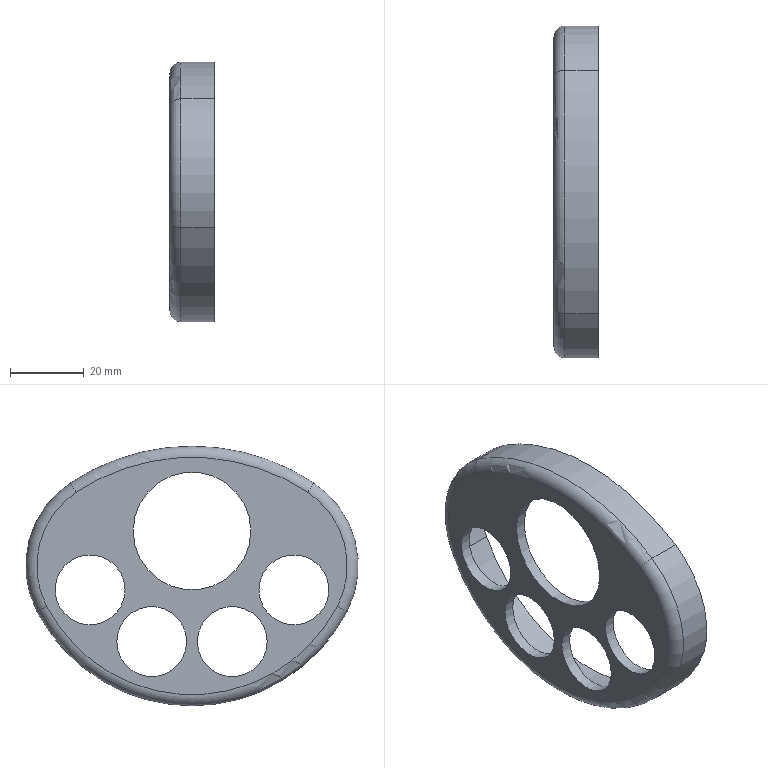Part | STEP file | 1-57.2 | 1 solid | 20 faces | box 12 x 90.4 x 70.538 mm | volume 15171 mm3 | cylinder 13 | torus 4 | plane 3 | commonest cylinder face diameters 19 x4 48 x2 54 x2 32 x1 89 x1 95 x1